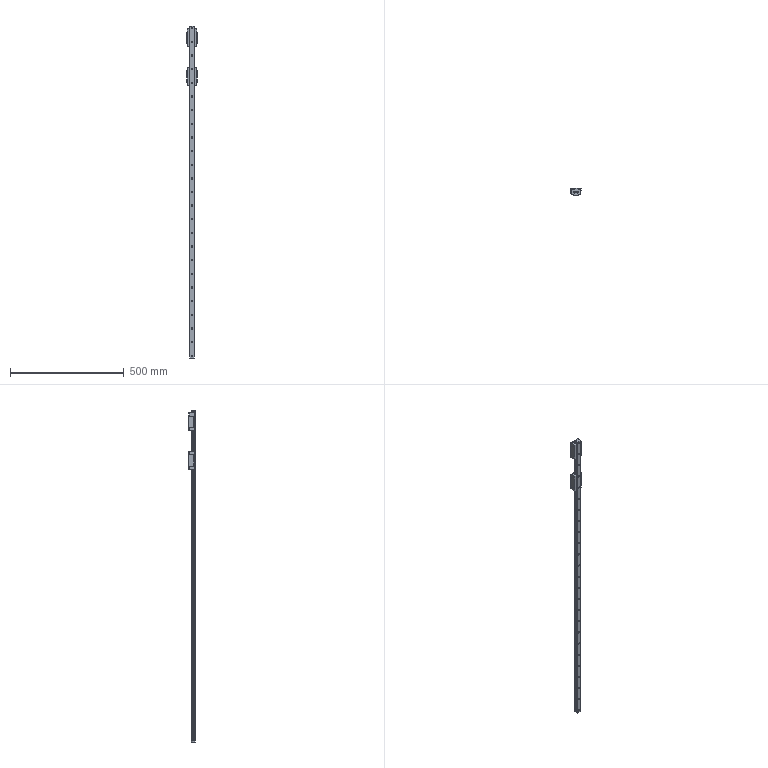Part | NX | 3 solids | 865 faces | box 44 x 30 x 1460 mm | volume 551478 mm3 | plane 617 | cylinder 128 | spline 120 | commonest cylinder face diameters 1 x36 6 x25 10 x25 2 x22 4.06 x12 5 x8